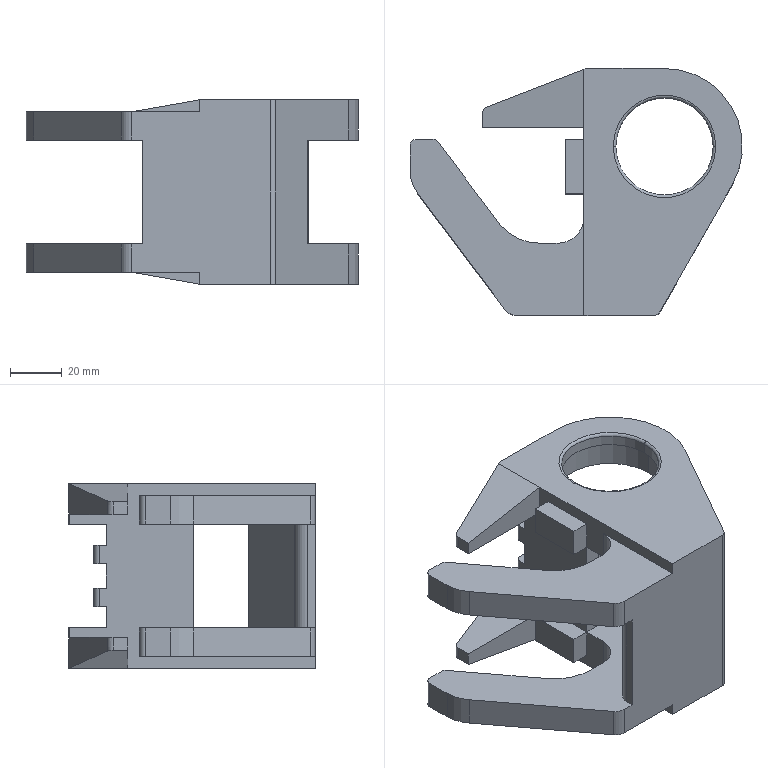Part | STEP file | 1 solid | 95 faces | box 128 x 95 x 71 mm | volume 210049 mm3 | plane 57 | cylinder 34 | torus 4 | commonest cylinder face diameters 5 x8 4 x4 37.5 x4 42 x4 10 x3 20 x2